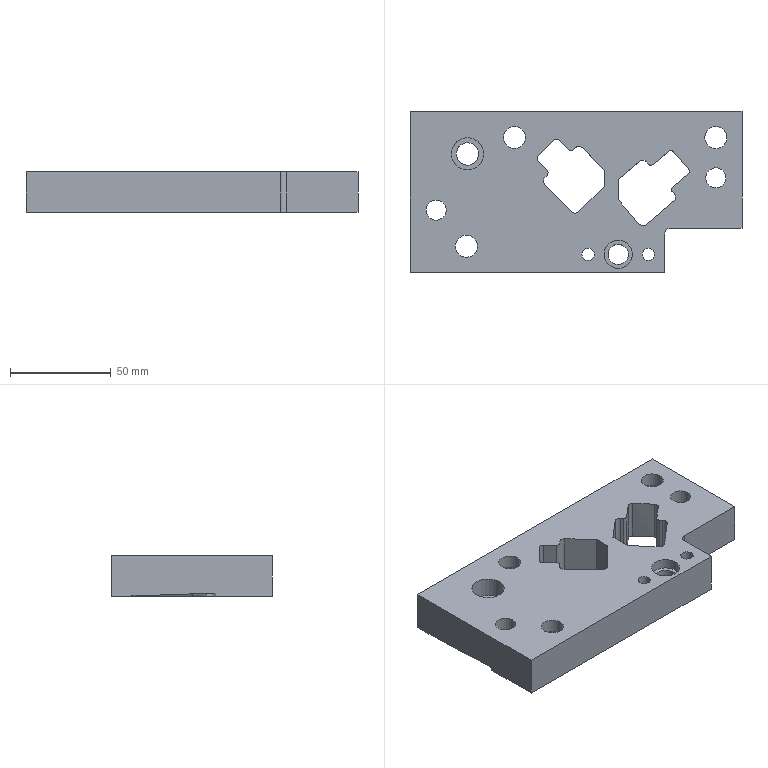Part | STEP file | 430_id2786_x_t | 1 solid | 76 faces | box 165 x 80 x 20 mm | volume 194228 mm3 | plane 33 | cylinder 31 | spline 12 | commonest cylinder face diameters 5 x6 11 x5 3 x4 4 x4 10 x3 17 x3